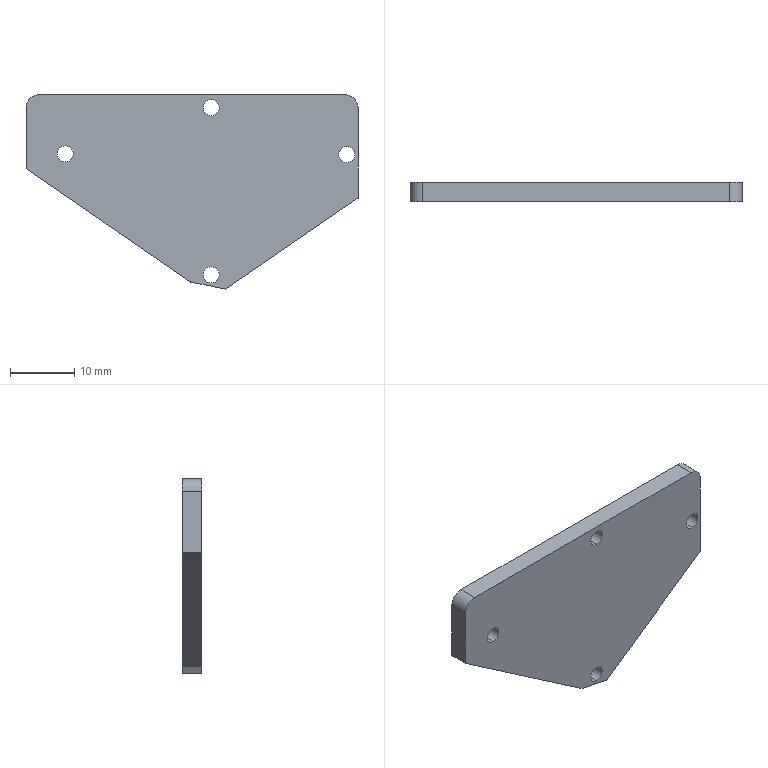Part | SolidWorks | features ICE 4, Fillet 2, Cut 1, Extrusion 1, MoveFace 1 | 1 solid | 20 faces | box 51.5 x 3 x 30.146 mm | volume 3390 mm3 | cylinder 10 | plane 10 | commonest cylinder face diameters 2.5 x8 4 x2
STEP:
#1=CARTESIAN_POINT('',(41.25,0.,-7.573));
#2=VERTEX_POINT('',#1);
#3=CARTESIAN_POINT('',(41.25,0.,-5.073));
#4=VERTEX_POINT('',#3);
#5=CARTESIAN_POINT('',(41.25,0.,-6.323));
#6=DIRECTION('',(0.,1.,0.));
#7=DIRECTION('',(0.,0.,1.));
#8=AXIS2_PLACEMENT_3D('',#5,#6,#7);
#9=CIRCLE('',#8,1.25);
#10=EDGE_CURVE('',#2,#4,#9,.T.);
#11=ORIENTED_EDGE('',*,*,#10,.F.);
#12=CARTESIAN_POINT('',(41.25,3.,-7.573));
#13=VERTEX_POINT('',#12);
#14=CARTESIAN_POINT('',(41.25,-6.,-7.573));
#15=DIRECTION('',(0.,1.,0.));
#16=VECTOR('',#15,1000.);
#17=LINE('',#14,#16);
#18=EDGE_CURVE('',#2,#13,#17,.T.);
#19=ORIENTED_EDGE('',*,*,#18,.T.);
#20=CARTESIAN_POINT('',(41.25,3.,-5.073));
#21=VERTEX_POINT('',#20);
#22=CARTESIAN_POINT('',(41.25,3.,-6.323));
#23=DIRECTION('',(0.,1.,0.));
#24=DIRECTION('',(0.,0.,1.));
#25=AXIS2_PLACEMENT_3D('',#22,#23,#24);
#26=CIRCLE('',#25,1.25);
#27=EDGE_CURVE('',#13,#21,#26,.T.);
#28=ORIENTED_EDGE('',*,*,#27,.T.);
#29=CARTESIAN_POINT('',(41.25,-6.,-5.073));
#30=DIRECTION('',(0.,1.,0.));
#31=VECTOR('',#30,1000.);
#32=LINE('',#29,#31);
#33=EDGE_CURVE('',#4,#21,#32,.T.);
#34=ORIENTED_EDGE('',*,*,#33,.F.);
#35=EDGE_LOOP('',(#11,#19,#28,#34));
#36=FACE_OUTER_BOUND('',#35,.T.);
#37=CARTESIAN_POINT('',(41.25,-6.,-6.323));
#38=DIRECTION('',(0.,1.,0.));
#39=DIRECTION('',(0.,0.,1.));
#40=AXIS2_PLACEMENT_3D('',#37,#38,#39);
#41=CYLINDRICAL_SURFACE('',#40,1.25);
#42=ADVANCED_FACE('',(#36),#41,.F.);
#43=CARTESIAN_POINT('',(20.25,0.,-0.2727));
#44=VERTEX_POINT('',#43);
#45=CARTESIAN_POINT('',(20.25,0.,2.227));
#46=VERTEX_POINT('',#45);
#47=CARTESIAN_POINT('',(20.25,0.,0.9773));
#48=DIRECTION('',(0.,1.,0.));
#49=DIRECTION('',(0.,0.,1.));
#50=AXIS2_PLACEMENT_3D('',#47,#48,#49);
#51=CIRCLE('',#50,1.25);
#52=EDGE_CURVE('',#44,#46,#51,.T.);
#53=ORIENTED_EDGE('',*,*,#52,.F.);
#54=CARTESIAN_POINT('',(20.25,3.,-0.2727));
#55=VERTEX_POINT('',#54);
#56=CARTESIAN_POINT('',(20.25,-6.,-0.2727));
#57=DIRECTION('',(0.,1.,0.));
#58=VECTOR('',#57,1000.);
#59=LINE('',#56,#58);
#60=EDGE_CURVE('',#44,#55,#59,.T.);
#61=ORIENTED_EDGE('',*,*,#60,.T.);
#62=CARTESIAN_POINT('',(20.25,3.,2.227));
#63=VERTEX_POINT('',#62);
#64=CARTESIAN_POINT('',(20.25,3.,0.9773));
#65=DIRECTION('',(0.,1.,0.));
#66=DIRECTION('',(0.,0.,1.));
#67=AXIS2_PLACEMENT_3D('',#64,#65,#66);
#68=CIRCLE('',#67,1.25);
#69=EDGE_CURVE('',#55,#63,#68,.T.);
#70=ORIENTED_EDGE('',*,*,#69,.T.);
#71=CARTESIAN_POINT('',(20.25,-6.,2.227));
#72=DIRECTION('',(0.,1.,0.));
#73=VECTOR('',#72,1000.);
#74=LINE('',#71,#73);
#75=EDGE_CURVE('',#46,#63,#74,.T.);
#76=ORIENTED_EDGE('',*,*,#75,.F.);
#77=EDGE_LOOP('',(#53,#61,#70,#76));
#78=FACE_OUTER_BOUND('',#77,.T.);
#79=CARTESIAN_POINT('',(20.25,-6.,0.9773));
#80=DIRECTION('',(0.,1.,0.));
#81=DIRECTION('',(0.,0.,1.));
#82=AXIS2_PLACEMENT_3D('',#79,#80,#81);
#83=CYLINDRICAL_SURFACE('',#82,1.25);
#84=ADVANCED_FACE('',(#78),#83,.F.);
#85=CARTESIAN_POINT('',(-2.398,0.,-7.437));
#86=VERTEX_POINT('',#85);
#87=CARTESIAN_POINT('',(-2.398,0.,-4.937));
#88=VERTEX_POINT('',#87);
#89=CARTESIAN_POINT('',(-2.398,0.,-6.187));
#90=DIRECTION('',(0.,1.,0.));
#91=DIRECTION('',(0.,0.,1.));
#92=AXIS2_PLACEMENT_3D('',#89,#90,#91);
#93=CIRCLE('',#92,1.25);
#94=EDGE_CURVE('',#86,#88,#93,.T.);
#95=ORIENTED_EDGE('',*,*,#94,.F.);
#96=CARTESIAN_POINT('',(-2.398,3.,-7.437));
#97=VERTEX_POINT('',#96);
#98=CARTESIAN_POINT('',(-2.398,-6.,-7.437));
#99=DIRECTION('',(0.,1.,0.));
#100=VECTOR('',#99,1000.);
#101=LINE('',#98,#100);
#102=EDGE_CURVE('',#86,#97,#101,.T.);
#103=ORIENTED_EDGE('',*,*,#102,.T.);
#104=CARTESIAN_POINT('',(-2.398,3.,-4.937));
#105=VERTEX_POINT('',#104);
#106=CARTESIAN_POINT('',(-2.398,3.,-6.187));
#107=DIRECTION('',(0.,1.,0.));
#108=DIRECTION('',(0.,0.,1.));
#109=AXIS2_PLACEMENT_3D('',#106,#107,#108);
#110=CIRCLE('',#109,1.25);
#111=EDGE_CURVE('',#97,#105,#110,.T.);
#112=ORIENTED_EDGE('',*,*,#111,.T.);
#113=CARTESIAN_POINT('',(-2.398,-6.,-4.937));
#114=DIRECTION('',(0.,1.,0.));
#115=VECTOR('',#114,1000.);
#116=LINE('',#113,#115);
#117=EDGE_CURVE('',#88,#105,#116,.T.);
#118=ORIENTED_EDGE('',*,*,#117,.F.);
#119=EDGE_LOOP('',(#95,#103,#112,#118));
#120=FACE_OUTER_BOUND('',#119,.T.);
#121=CARTESIAN_POINT('',(-2.398,-6.,-6.187));
#122=DIRECTION('',(0.,1.,0.));
#123=DIRECTION('',(0.,0.,1.));
#124=AXIS2_PLACEMENT_3D('',#121,#122,#123);
#125=CYLINDRICAL_SURFACE('',#124,1.25);
#126=ADVANCED_FACE('',(#120),#125,.F.);
#127=CARTESIAN_POINT('',(20.25,0.,-26.2));
#128=VERTEX_POINT('',#127);
#129=CARTESIAN_POINT('',(20.25,0.,-23.7));
#130=VERTEX_POINT('',#129);
#131=CARTESIAN_POINT('',(20.25,0.,-24.95));
#132=DIRECTION('',(0.,1.,0.));
#133=DIRECTION('',(0.,0.,1.));
#134=AXIS2_PLACEMENT_3D('',#131,#132,#133);
#135=CIRCLE('',#134,1.25);
#136=EDGE_CURVE('',#128,#130,#135,.T.);
#137=ORIENTED_EDGE('',*,*,#136,.F.);
#138=CARTESIAN_POINT('',(20.25,3.,-26.2));
#139=VERTEX_POINT('',#138);
#140=CARTESIAN_POINT('',(20.25,0.,-26.2));
#141=DIRECTION('',(0.,1.,0.));
#142=VECTOR('',#141,1000.);
#143=LINE('',#140,#142);
#144=EDGE_CURVE('',#128,#139,#143,.T.);
#145=ORIENTED_EDGE('',*,*,#144,.T.);
#146=CARTESIAN_POINT('',(20.25,3.,-23.7));
#147=VERTEX_POINT('',#146);
#148=CARTESIAN_POINT('',(20.25,3.,-24.95));
#149=DIRECTION('',(0.,1.,0.));
#150=DIRECTION('',(0.,0.,1.));
#151=AXIS2_PLACEMENT_3D('',#148,#149,#150);
#152=CIRCLE('',#151,1.25);
#153=EDGE_CURVE('',#139,#147,#152,.T.);
#154=ORIENTED_EDGE('',*,*,#153,.T.);
#155=CARTESIAN_POINT('',(20.25,0.,-23.7));
#156=DIRECTION('',(0.,1.,0.));
#157=VECTOR('',#156,1000.);
#158=LINE('',#155,#157);
#159=EDGE_CURVE('',#130,#147,#158,.T.);
#160=ORIENTED_EDGE('',*,*,#159,.F.);
#161=EDGE_LOOP('',(#137,#145,#154,#160));
#162=FACE_OUTER_BOUND('',#161,.T.);
#163=CARTESIAN_POINT('',(20.25,0.,-24.95));
#164=DIRECTION('',(0.,1.,0.));
#165=DIRECTION('',(0.,0.,1.));
#166=AXIS2_PLACEMENT_3D('',#163,#164,#165);
#167=CYLINDRICAL_SURFACE('',#166,1.25);
#168=ADVANCED_FACE('',(#162),#167,.F.);
#169=CARTESIAN_POINT('',(41.25,3.,-6.323));
#170=DIRECTION('',(0.,1.,0.));
#171=DIRECTION('',(0.,0.,1.));
#172=AXIS2_PLACEMENT_3D('',#169,#170,#171);
#173=CIRCLE('',#172,1.25);
#174=EDGE_CURVE('',#21,#13,#173,.T.);
#175=ORIENTED_EDGE('',*,*,#174,.F.);
#176=ORIENTED_EDGE('',*,*,#27,.F.);
#177=EDGE_LOOP('',(#175,#176));
#178=FACE_BOUND('',#177,.T.);
#179=CARTESIAN_POINT('',(20.25,3.,0.9773));
#180=DIRECTION('',(0.,1.,0.));
#181=DIRECTION('',(0.,0.,1.));
#182=AXIS2_PLACEMENT_3D('',#179,#180,#181);
#183=CIRCLE('',#182,1.25);
#184=EDGE_CURVE('',#63,#55,#183,.T.);
#185=ORIENTED_EDGE('',*,*,#184,.F.);
#186=ORIENTED_EDGE('',*,*,#69,.F.);
#187=EDGE_LOOP('',(#185,#186));
#188=FACE_BOUND('',#187,.T.);
#189=CARTESIAN_POINT('',(-2.398,3.,-6.187));
#190=DIRECTION('',(0.,1.,0.));
#191=DIRECTION('',(0.,0.,1.));
#192=AXIS2_PLACEMENT_3D('',#189,#190,#191);
#193=CIRCLE('',#192,1.25);
#194=EDGE_CURVE('',#105,#97,#193,.T.);
#195=ORIENTED_EDGE('',*,*,#194,.F.);
#196=ORIENTED_EDGE('',*,*,#111,.F.);
#197=EDGE_LOOP('',(#195,#196));
#198=FACE_BOUND('',#197,.T.);
#199=CARTESIAN_POINT('',(43.,3.,-13.049));
#200=VERTEX_POINT('',#199);
#201=CARTESIAN_POINT('',(42.96,3.,-13.054));
#202=VERTEX_POINT('',#201);
#203=CARTESIAN_POINT('',(17.067,3.,-16.182));
#204=DIRECTION('',(-0.9928,0.,-0.1199));
#205=VECTOR('',#204,1000.);
#206=LINE('',#203,#205);
#207=EDGE_CURVE('',#200,#202,#206,.T.);
#208=ORIENTED_EDGE('',*,*,#207,.T.);
#209=CARTESIAN_POINT('',(22.422,3.,-27.169));
#210=VERTEX_POINT('',#209);
#211=CARTESIAN_POINT('',(22.422,3.,-27.169));
#212=DIRECTION('',(0.8241,0.,0.5664));
#213=VECTOR('',#212,1000.);
#214=LINE('',#211,#213);
#215=EDGE_CURVE('',#210,#202,#214,.T.);
#216=ORIENTED_EDGE('',*,*,#215,.F.);
#217=CARTESIAN_POINT('',(17.067,3.,-26.05));
#218=VERTEX_POINT('',#217);
#219=CARTESIAN_POINT('',(17.067,3.,-26.05));
#220=DIRECTION('',(0.9789,0.,-0.2046));
#221=VECTOR('',#220,1000.);
#222=LINE('',#219,#221);
#223=EDGE_CURVE('',#218,#210,#222,.T.);
#224=ORIENTED_EDGE('',*,*,#223,.F.);
#225=CARTESIAN_POINT('',(17.067,3.,-26.073));
#226=VERTEX_POINT('',#225);
#227=CARTESIAN_POINT('',(17.067,3.,-26.073));
#228=DIRECTION('',(0.,0.,-1.));
#229=VECTOR('',#228,1000.);
#230=LINE('',#227,#229);
#231=EDGE_CURVE('',#218,#226,#230,.T.);
#232=ORIENTED_EDGE('',*,*,#231,.T.);
#233=CARTESIAN_POINT('',(-8.5,3.,-8.501));
#234=VERTEX_POINT('',#233);
#235=CARTESIAN_POINT('',(-8.5,3.,-8.501));
#236=DIRECTION('',(-0.8241,0.,0.5664));
#237=VECTOR('',#236,1000.);
#238=LINE('',#235,#237);
#239=EDGE_CURVE('',#226,#234,#238,.T.);
#240=ORIENTED_EDGE('',*,*,#239,.T.);
#241=CARTESIAN_POINT('',(-8.5,3.,0.9773));
#242=VERTEX_POINT('',#241);
#243=CARTESIAN_POINT('',(-8.5,3.,0.9773));
#244=DIRECTION('',(0.,0.,1.));
#245=VECTOR('',#244,1000.);
#246=LINE('',#243,#245);
#247=EDGE_CURVE('',#234,#242,#246,.T.);
#248=ORIENTED_EDGE('',*,*,#247,.T.);
#249=CARTESIAN_POINT('',(-6.5,3.,2.977));
#250=VERTEX_POINT('',#249);
#251=CARTESIAN_POINT('',(-6.5,3.,0.9773));
#252=DIRECTION('',(0.,1.,0.));
#253=DIRECTION('',(0.,0.,1.));
#254=AXIS2_PLACEMENT_3D('',#251,#252,#253);
#255=CIRCLE('',#254,2.);
#256=EDGE_CURVE('',#242,#250,#255,.T.);
#257=ORIENTED_EDGE('',*,*,#256,.T.);
#258=CARTESIAN_POINT('',(41.,3.,2.977));
#259=VERTEX_POINT('',#258);
#260=CARTESIAN_POINT('',(41.,3.,2.977));
#261=DIRECTION('',(1.,0.,0.));
#262=VECTOR('',#261,1000.);
#263=LINE('',#260,#262);
#264=EDGE_CURVE('',#250,#259,#263,.T.);
#265=ORIENTED_EDGE('',*,*,#264,.T.);
#266=CARTESIAN_POINT('',(43.,3.,0.9773));
#267=VERTEX_POINT('',#266);
#268=CARTESIAN_POINT('',(41.,3.,0.9773));
#269=DIRECTION('',(0.,1.,0.));
#270=DIRECTION('',(0.,0.,1.));
#271=AXIS2_PLACEMENT_3D('',#268,#269,#270);
#272=CIRCLE('',#271,2.);
#273=EDGE_CURVE('',#259,#267,#272,.T.);
#274=ORIENTED_EDGE('',*,*,#273,.T.);
#275=CARTESIAN_POINT('',(43.,3.,-13.026));
#276=DIRECTION('',(0.,0.,-1.));
#277=VECTOR('',#276,1000.);
#278=LINE('',#275,#277);
#279=EDGE_CURVE('',#267,#200,#278,.T.);
#280=ORIENTED_EDGE('',*,*,#279,.T.);
#281=EDGE_LOOP('',(#208,#216,#224,#232,#240,#248,#257,#265,#274,#280));
#282=FACE_OUTER_BOUND('',#281,.T.);
#283=CARTESIAN_POINT('',(20.25,3.,-24.95));
#284=DIRECTION('',(0.,1.,0.));
#285=DIRECTION('',(0.,0.,1.));
#286=AXIS2_PLACEMENT_3D('',#283,#284,#285);
#287=CIRCLE('',#286,1.25);
#288=EDGE_CURVE('',#147,#139,#287,.T.);
#289=ORIENTED_EDGE('',*,*,#288,.F.);
#290=ORIENTED_EDGE('',*,*,#153,.F.);
#291=EDGE_LOOP('',(#289,#290));
#292=FACE_BOUND('',#291,.T.);
#293=CARTESIAN_POINT('',(0.,3.,0.));
#294=DIRECTION('',(0.,1.,0.));
#295=DIRECTION('',(0.,0.,1.));
#296=AXIS2_PLACEMENT_3D('',#293,#294,#295);
#297=PLANE('',#296);
#298=ADVANCED_FACE('',(#178,#188,#198,#282,#292),#297,.T.);
#299=CARTESIAN_POINT('',(41.25,0.,-6.323));
#300=DIRECTION('',(0.,1.,0.));
#301=DIRECTION('',(0.,0.,1.));
#302=AXIS2_PLACEMENT_3D('',#299,#300,#301);
#303=CIRCLE('',#302,1.25);
#304=EDGE_CURVE('',#4,#2,#303,.T.);
#305=ORIENTED_EDGE('',*,*,#304,.T.);
#306=ORIENTED_EDGE('',*,*,#10,.T.);
#307=EDGE_LOOP('',(#305,#306));
#308=FACE_BOUND('',#307,.T.);
#309=CARTESIAN_POINT('',(20.25,0.,0.9773));
#310=DIRECTION('',(0.,1.,0.));
#311=DIRECTION('',(0.,0.,1.));
#312=AXIS2_PLACEMENT_3D('',#309,#310,#311);
#313=CIRCLE('',#312,1.25);
#314=EDGE_CURVE('',#46,#44,#313,.T.);
#315=ORIENTED_EDGE('',*,*,#314,.T.);
#316=ORIENTED_EDGE('',*,*,#52,.T.);
#317=EDGE_LOOP('',(#315,#316));
#318=FACE_BOUND('',#317,.T.);
#319=CARTESIAN_POINT('',(-2.398,0.,-6.187));
#320=DIRECTION('',(0.,1.,0.));
#321=DIRECTION('',(0.,0.,1.));
#322=AXIS2_PLACEMENT_3D('',#319,#320,#321);
#323=CIRCLE('',#322,1.25);
#324=EDGE_CURVE('',#88,#86,#323,.T.);
#325=ORIENTED_EDGE('',*,*,#324,.T.);
#326=ORIENTED_EDGE('',*,*,#94,.T.);
#327=EDGE_LOOP('',(#325,#326));
#328=FACE_BOUND('',#327,.T.);
#329=CARTESIAN_POINT('',(20.25,0.,-24.95));
#330=DIRECTION('',(0.,1.,0.));
#331=DIRECTION('',(0.,0.,1.));
#332=AXIS2_PLACEMENT_3D('',#329,#330,#331);
#333=CIRCLE('',#332,1.25);
#334=EDGE_CURVE('',#130,#128,#333,.T.);
#335=ORIENTED_EDGE('',*,*,#334,.T.);
#336=ORIENTED_EDGE('',*,*,#136,.T.);
#337=EDGE_LOOP('',(#335,#336));
#338=FACE_BOUND('',#337,.T.);
#339=CARTESIAN_POINT('',(22.422,0.,-27.169));
#340=VERTEX_POINT('',#339);
#341=CARTESIAN_POINT('',(42.96,0.,-13.054));
#342=VERTEX_POINT('',#341);
#343=CARTESIAN_POINT('',(22.422,0.,-27.169));
#344=DIRECTION('',(0.8241,0.,0.5664));
#345=VECTOR('',#344,1000.);
#346=LINE('',#343,#345);
#347=EDGE_CURVE('',#340,#342,#346,.T.);
#348=ORIENTED_EDGE('',*,*,#347,.T.);
#349=CARTESIAN_POINT('',(43.,0.,-13.049));
#350=VERTEX_POINT('',#349);
#351=CARTESIAN_POINT('',(17.067,0.,-16.182));
#352=DIRECTION('',(0.9928,0.,0.1199));
#353=VECTOR('',#352,1000.);
#354=LINE('',#351,#353);
#355=EDGE_CURVE('',#342,#350,#354,.T.);
#356=ORIENTED_EDGE('',*,*,#355,.T.);
#357=CARTESIAN_POINT('',(43.,0.,0.9773));
#358=VERTEX_POINT('',#357);
#359=CARTESIAN_POINT('',(43.,0.,-13.026));
#360=DIRECTION('',(0.,0.,-1.));
#361=VECTOR('',#360,1000.);
#362=LINE('',#359,#361);
#363=EDGE_CURVE('',#358,#350,#362,.T.);
#364=ORIENTED_EDGE('',*,*,#363,.F.);
#365=CARTESIAN_POINT('',(41.,0.,2.977));
#366=VERTEX_POINT('',#365);
#367=CARTESIAN_POINT('',(41.,0.,0.9773));
#368=DIRECTION('',(0.,-1.,0.));
#369=DIRECTION('',(0.,0.,1.));
#370=AXIS2_PLACEMENT_3D('',#367,#368,#369);
#371=CIRCLE('',#370,2.);
#372=EDGE_CURVE('',#358,#366,#371,.T.);
#373=ORIENTED_EDGE('',*,*,#372,.T.);
#374=CARTESIAN_POINT('',(-6.5,0.,2.977));
#375=VERTEX_POINT('',#374);
#376=CARTESIAN_POINT('',(41.,0.,2.977));
#377=DIRECTION('',(-1.,0.,0.));
#378=VECTOR('',#377,1000.);
#379=LINE('',#376,#378);
#380=EDGE_CURVE('',#366,#375,#379,.T.);
#381=ORIENTED_EDGE('',*,*,#380,.T.);
#382=CARTESIAN_POINT('',(-8.5,0.,0.9773));
#383=VERTEX_POINT('',#382);
#384=CARTESIAN_POINT('',(-6.5,0.,0.9773));
#385=DIRECTION('',(0.,-1.,0.));
#386=DIRECTION('',(0.,0.,1.));
#387=AXIS2_PLACEMENT_3D('',#384,#385,#386);
#388=CIRCLE('',#387,2.);
#389=EDGE_CURVE('',#375,#383,#388,.T.);
#390=ORIENTED_EDGE('',*,*,#389,.T.);
#391=CARTESIAN_POINT('',(-8.5,0.,-8.501));
#392=VERTEX_POINT('',#391);
#393=CARTESIAN_POINT('',(-8.5,0.,0.9773));
#394=DIRECTION('',(0.,0.,-1.));
#395=VECTOR('',#394,1000.);
#396=LINE('',#393,#395);
#397=EDGE_CURVE('',#383,#392,#396,.T.);
#398=ORIENTED_EDGE('',*,*,#397,.T.);
#399=CARTESIAN_POINT('',(17.067,0.,-26.073));
#400=VERTEX_POINT('',#399);
#401=CARTESIAN_POINT('',(-8.5,0.,-8.501));
#402=DIRECTION('',(0.8241,0.,-0.5664));
#403=VECTOR('',#402,1000.);
#404=LINE('',#401,#403);
#405=EDGE_CURVE('',#392,#400,#404,.T.);
#406=ORIENTED_EDGE('',*,*,#405,.T.);
#407=CARTESIAN_POINT('',(17.067,0.,-26.05));
#408=VERTEX_POINT('',#407);
#409=CARTESIAN_POINT('',(17.067,0.,-26.073));
#410=DIRECTION('',(0.,0.,1.));
#411=VECTOR('',#410,1000.);
#412=LINE('',#409,#411);
#413=EDGE_CURVE('',#400,#408,#412,.T.);
#414=ORIENTED_EDGE('',*,*,#413,.T.);
#415=CARTESIAN_POINT('',(17.067,0.,-26.05));
#416=DIRECTION('',(0.9789,0.,-0.2046));
#417=VECTOR('',#416,1000.);
#418=LINE('',#415,#417);
#419=EDGE_CURVE('',#408,#340,#418,.T.);
#420=ORIENTED_EDGE('',*,*,#419,.T.);
#421=EDGE_LOOP('',(#348,#356,#364,#373,#381,#390,#398,#406,#414,#420));
#422=FACE_OUTER_BOUND('',#421,.T.);
#423=CARTESIAN_POINT('',(0.,0.,0.));
#424=DIRECTION('',(0.,1.,0.));
#425=DIRECTION('',(0.,0.,1.));
#426=AXIS2_PLACEMENT_3D('',#423,#424,#425);
#427=PLANE('',#426);
#428=ADVANCED_FACE('',(#308,#318,#328,#338,#422),#427,.F.);
#429=ORIENTED_EDGE('',*,*,#215,.T.);
#430=CARTESIAN_POINT('',(42.96,0.,-13.054));
#431=DIRECTION('',(0.,-1.,0.));
#432=VECTOR('',#431,1000.);
#433=LINE('',#430,#432);
#434=EDGE_CURVE('',#202,#342,#433,.T.);
#435=ORIENTED_EDGE('',*,*,#434,.T.);
#436=ORIENTED_EDGE('',*,*,#347,.F.);
#437=CARTESIAN_POINT('',(22.422,0.,-27.169));
#438=DIRECTION('',(0.,1.,0.));
#439=VECTOR('',#438,1000.);
#440=LINE('',#437,#439);
#441=EDGE_CURVE('',#340,#210,#440,.T.);
#442=ORIENTED_EDGE('',*,*,#441,.T.);
#443=EDGE_LOOP('',(#429,#435,#436,#442));
#444=FACE_OUTER_BOUND('',#443,.T.);
#445=CARTESIAN_POINT('',(22.422,0.,-27.169));
#446=DIRECTION('',(-0.5664,0.,0.8241));
#447=DIRECTION('',(0.8241,0.,0.5664));
#448=AXIS2_PLACEMENT_3D('',#445,#446,#447);
#449=PLANE('',#448);
#450=ADVANCED_FACE('',(#444),#449,.F.);
#451=ORIENTED_EDGE('',*,*,#223,.T.);
#452=ORIENTED_EDGE('',*,*,#441,.F.);
#453=ORIENTED_EDGE('',*,*,#419,.F.);
#454=CARTESIAN_POINT('',(17.067,0.,-26.05));
#455=DIRECTION('',(0.,1.,0.));
#456=VECTOR('',#455,1000.);
#457=LINE('',#454,#456);
#458=EDGE_CURVE('',#408,#218,#457,.T.);
#459=ORIENTED_EDGE('',*,*,#458,.T.);
#460=EDGE_LOOP('',(#451,#452,#453,#459));
#461=FACE_OUTER_BOUND('',#460,.T.);
#462=CARTESIAN_POINT('',(17.067,0.,-26.05));
#463=DIRECTION('',(0.2046,0.,0.9789));
#464=DIRECTION('',(0.9789,0.,-0.2046));
#465=AXIS2_PLACEMENT_3D('',#462,#463,#464);
#466=PLANE('',#465);
#467=ADVANCED_FACE('',(#461),#466,.F.);
#468=ORIENTED_EDGE('',*,*,#279,.F.);
#469=CARTESIAN_POINT('',(43.,-59.128,0.9773));
#470=DIRECTION('',(0.,1.,0.));
#471=VECTOR('',#470,1000.);
#472=LINE('',#469,#471);
#473=EDGE_CURVE('',#358,#267,#472,.T.);
#474=ORIENTED_EDGE('',*,*,#473,.F.);
#475=ORIENTED_EDGE('',*,*,#363,.T.);
#476=CARTESIAN_POINT('',(43.,-59.128,-13.049));
#477=DIRECTION('',(0.,1.,0.));
#478=VECTOR('',#477,1000.);
#479=LINE('',#476,#478);
#480=EDGE_CURVE('',#350,#200,#479,.T.);
#481=ORIENTED_EDGE('',*,*,#480,.T.);
#482=EDGE_LOOP('',(#468,#474,#475,#481));
#483=FACE_OUTER_BOUND('',#482,.T.);
#484=CARTESIAN_POINT('',(43.,0.,-13.026));
#485=DIRECTION('',(1.,0.,0.));
#486=DIRECTION('',(0.,0.,-1.));
#487=AXIS2_PLACEMENT_3D('',#484,#485,#486);
#488=PLANE('',#487);
#489=ADVANCED_FACE('',(#483),#488,.T.);
#490=ORIENTED_EDGE('',*,*,#144,.F.);
#491=ORIENTED_EDGE('',*,*,#334,.F.);
#492=ORIENTED_EDGE('',*,*,#159,.T.);
#493=ORIENTED_EDGE('',*,*,#288,.T.);
#494=EDGE_LOOP('',(#490,#491,#492,#493));
#495=FACE_OUTER_BOUND('',#494,.T.);
#496=CARTESIAN_POINT('',(20.25,0.,-24.95));
#497=DIRECTION('',(0.,1.,0.));
#498=DIRECTION('',(0.,0.,1.));
#499=AXIS2_PLACEMENT_3D('',#496,#497,#498);
#500=CYLINDRICAL_SURFACE('',#499,1.25);
#501=ADVANCED_FACE('',(#495),#500,.F.);
#502=ORIENTED_EDGE('',*,*,#405,.F.);
#503=CARTESIAN_POINT('',(-8.5,-59.128,-8.501));
#504=DIRECTION('',(0.,1.,0.));
#505=VECTOR('',#504,1000.);
#506=LINE('',#503,#505);
#507=EDGE_CURVE('',#392,#234,#506,.T.);
#508=ORIENTED_EDGE('',*,*,#507,.T.);
#509=ORIENTED_EDGE('',*,*,#239,.F.);
#510=CARTESIAN_POINT('',(17.067,-59.128,-26.073));
#511=DIRECTION('',(0.,1.,0.));
#512=VECTOR('',#511,1000.);
#513=LINE('',#510,#512);
#514=EDGE_CURVE('',#400,#226,#513,.T.);
#515=ORIENTED_EDGE('',*,*,#514,.F.);
#516=EDGE_LOOP('',(#502,#508,#509,#515));
#517=FACE_OUTER_BOUND('',#516,.T.);
#518=CARTESIAN_POINT('',(-8.5,-59.128,-8.501));
#519=DIRECTION('',(-0.5664,0.,-0.8241));
#520=DIRECTION('',(-0.8241,0.,0.5664));
#521=AXIS2_PLACEMENT_3D('',#518,#519,#520);
#522=PLANE('',#521);
#523=ADVANCED_FACE('',(#517),#522,.T.);
#524=ORIENTED_EDGE('',*,*,#397,.F.);
#525=CARTESIAN_POINT('',(-8.5,-59.128,0.9773));
#526=DIRECTION('',(0.,1.,0.));
#527=VECTOR('',#526,1000.);
#528=LINE('',#525,#527);
#529=EDGE_CURVE('',#383,#242,#528,.T.);
#530=ORIENTED_EDGE('',*,*,#529,.T.);
#531=ORIENTED_EDGE('',*,*,#247,.F.);
#532=ORIENTED_EDGE('',*,*,#507,.F.);
#533=EDGE_LOOP('',(#524,#530,#531,#532));
#534=FACE_OUTER_BOUND('',#533,.T.);
#535=CARTESIAN_POINT('',(-8.5,-59.128,0.9773));
#536=DIRECTION('',(-1.,0.,0.));
#537=DIRECTION('',(0.,0.,1.));
#538=AXIS2_PLACEMENT_3D('',#535,#536,#537);
#539=PLANE('',#538);
#540=ADVANCED_FACE('',(#534),#539,.T.);
#541=ORIENTED_EDGE('',*,*,#389,.F.);
#542=CARTESIAN_POINT('',(-6.5,-59.128,2.977));
#543=DIRECTION('',(0.,1.,0.));
#544=VECTOR('',#543,1000.);
#545=LINE('',#542,#544);
#546=EDGE_CURVE('',#375,#250,#545,.T.);
#547=ORIENTED_EDGE('',*,*,#546,.T.);
#548=ORIENTED_EDGE('',*,*,#256,.F.);
#549=ORIENTED_EDGE('',*,*,#529,.F.);
#550=EDGE_LOOP('',(#541,#547,#548,#549));
#551=FACE_OUTER_BOUND('',#550,.T.);
#552=CARTESIAN_POINT('',(-6.5,-59.128,0.9773));
#553=DIRECTION('',(0.,1.,0.));
#554=DIRECTION('',(0.,0.,1.));
#555=AXIS2_PLACEMENT_3D('',#552,#553,#554);
#556=CYLINDRICAL_SURFACE('',#555,2.);
#557=ADVANCED_FACE('',(#551),#556,.T.);
#558=ORIENTED_EDGE('',*,*,#380,.F.);
#559=CARTESIAN_POINT('',(41.,-59.128,2.977));
#560=DIRECTION('',(0.,1.,0.));
#561=VECTOR('',#560,1000.);
#562=LINE('',#559,#561);
#563=EDGE_CURVE('',#366,#259,#562,.T.);
#564=ORIENTED_EDGE('',*,*,#563,.T.);
#565=ORIENTED_EDGE('',*,*,#264,.F.);
#566=ORIENTED_EDGE('',*,*,#546,.F.);
#567=EDGE_LOOP('',(#558,#564,#565,#566));
#568=FACE_OUTER_BOUND('',#567,.T.);
#569=CARTESIAN_POINT('',(41.,-59.128,2.977));
#570=DIRECTION('',(0.,0.,1.));
#571=DIRECTION('',(1.,0.,0.));
#572=AXIS2_PLACEMENT_3D('',#569,#570,#571);
#573=PLANE('',#572);
#574=ADVANCED_FACE('',(#568),#573,.T.);
#575=ORIENTED_EDGE('',*,*,#372,.F.);
#576=ORIENTED_EDGE('',*,*,#473,.T.);
#577=ORIENTED_EDGE('',*,*,#273,.F.);
#578=ORIENTED_EDGE('',*,*,#563,.F.);
#579=EDGE_LOOP('',(#575,#576,#577,#578));
#580=FACE_OUTER_BOUND('',#579,.T.);
#581=CARTESIAN_POINT('',(41.,-59.128,0.9773));
#582=DIRECTION('',(0.,1.,0.));
#583=DIRECTION('',(0.,0.,1.));
#584=AXIS2_PLACEMENT_3D('',#581,#582,#583);
#585=CYLINDRICAL_SURFACE('',#584,2.);
#586=ADVANCED_FACE('',(#580),#585,.T.);
#587=ORIENTED_EDGE('',*,*,#458,.F.);
#588=ORIENTED_EDGE('',*,*,#413,.F.);
#589=ORIENTED_EDGE('',*,*,#514,.T.);
#590=ORIENTED_EDGE('',*,*,#231,.F.);
#591=EDGE_LOOP('',(#587,#588,#589,#590));
#592=FACE_OUTER_BOUND('',#591,.T.);
#593=CARTESIAN_POINT('',(17.067,-59.128,-26.073));
#594=DIRECTION('',(1.,0.,0.));
#595=DIRECTION('',(0.,0.,-1.));
#596=AXIS2_PLACEMENT_3D('',#593,#594,#595);
#597=PLANE('',#596);
#598=ADVANCED_FACE('',(#592),#597,.T.);
#599=ORIENTED_EDGE('',*,*,#434,.F.);
#600=ORIENTED_EDGE('',*,*,#207,.F.);
#601=ORIENTED_EDGE('',*,*,#480,.F.);
#602=ORIENTED_EDGE('',*,*,#355,.F.);
#603=EDGE_LOOP('',(#599,#600,#601,#602));
#604=FACE_OUTER_BOUND('',#603,.T.);
#605=CARTESIAN_POINT('',(17.067,-59.128,-16.182));
#606=DIRECTION('',(0.1199,0.,-0.9928));
#607=DIRECTION('',(-0.9928,0.,-0.1199));
#608=AXIS2_PLACEMENT_3D('',#605,#606,#607);
#609=PLANE('',#608);
#610=ADVANCED_FACE('',(#604),#609,.T.);
#611=ORIENTED_EDGE('',*,*,#102,.F.);
#612=ORIENTED_EDGE('',*,*,#324,.F.);
#613=ORIENTED_EDGE('',*,*,#117,.T.);
#614=ORIENTED_EDGE('',*,*,#194,.T.);
#615=EDGE_LOOP('',(#611,#612,#613,#614));
#616=FACE_OUTER_BOUND('',#615,.T.);
#617=CARTESIAN_POINT('',(-2.398,-6.,-6.187));
#618=DIRECTION('',(0.,1.,0.));
#619=DIRECTION('',(0.,0.,1.));
#620=AXIS2_PLACEMENT_3D('',#617,#618,#619);
#621=CYLINDRICAL_SURFACE('',#620,1.25);
#622=ADVANCED_FACE('',(#616),#621,.F.);
#623=ORIENTED_EDGE('',*,*,#60,.F.);
#624=ORIENTED_EDGE('',*,*,#314,.F.);
#625=ORIENTED_EDGE('',*,*,#75,.T.);
#626=ORIENTED_EDGE('',*,*,#184,.T.);
#627=EDGE_LOOP('',(#623,#624,#625,#626));
#628=FACE_OUTER_BOUND('',#627,.T.);
#629=CARTESIAN_POINT('',(20.25,-6.,0.9773));
#630=DIRECTION('',(0.,1.,0.));
#631=DIRECTION('',(0.,0.,1.));
#632=AXIS2_PLACEMENT_3D('',#629,#630,#631);
#633=CYLINDRICAL_SURFACE('',#632,1.25);
#634=ADVANCED_FACE('',(#628),#633,.F.);
#635=ORIENTED_EDGE('',*,*,#18,.F.);
#636=ORIENTED_EDGE('',*,*,#304,.F.);
#637=ORIENTED_EDGE('',*,*,#33,.T.);
#638=ORIENTED_EDGE('',*,*,#174,.T.);
#639=EDGE_LOOP('',(#635,#636,#637,#638));
#640=FACE_OUTER_BOUND('',#639,.T.);
#641=CARTESIAN_POINT('',(41.25,-6.,-6.323));
#642=DIRECTION('',(0.,1.,0.));
#643=DIRECTION('',(0.,0.,1.));
#644=AXIS2_PLACEMENT_3D('',#641,#642,#643);
#645=CYLINDRICAL_SURFACE('',#644,1.25);
#646=ADVANCED_FACE('',(#640),#645,.F.);
#647=CLOSED_SHELL('',(#42,#84,#126,#168,#298,#428,#450,#467,#489,#501,#523,#540,#557,#574,#586,#598,#610,#622,#634,#646));
#648=MANIFOLD_SOLID_BREP('',#647);
#649=CARTESIAN_POINT('',(0.,0.,0.));
#650=DIRECTION('',(0.,0.,1.));
#651=DIRECTION('',(1.,0.,0.));
#652=AXIS2_PLACEMENT_3D('',#649,#650,#651);
#653=(LENGTH_UNIT()NAMED_UNIT(*)SI_UNIT(.MILLI.,.METRE.));
#654=UNCERTAINTY_MEASURE_WITH_UNIT(LENGTH_MEASURE(0.00001),#653,'','');
#655=(NAMED_UNIT(*)PLANE_ANGLE_UNIT()SI_UNIT($,.RADIAN.));
#656=(NAMED_UNIT(*)SI_UNIT($,.STERADIAN.)SOLID_ANGLE_UNIT());
#657=(GEOMETRIC_REPRESENTATION_CONTEXT(3)GLOBAL_UNCERTAINTY_ASSIGNED_CONTEXT((#654))GLOBAL_UNIT_ASSIGNED_CONTEXT((#653,#655,#656))REPRESENTATION_CONTEXT('',''));
#658=ADVANCED_BREP_SHAPE_REPRESENTATION('',(#648,#652),#657);